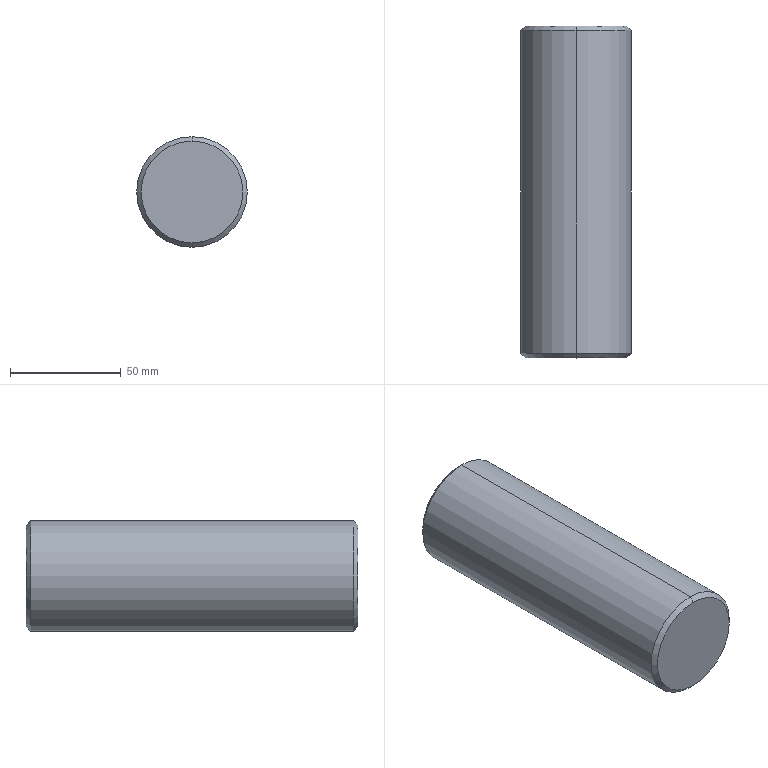Part | SolidWorks | 1 solid | 8 faces | box 50 x 150 x 50 mm | volume 293913 mm3 | cone 4 | cylinder 2 | plane 2 | commonest cylinder face diameters 50 x2
STEP:
#1=CARTESIAN_POINT('',(0.,0.,-23.));
#2=VERTEX_POINT('',#1);
#3=CARTESIAN_POINT('',(0.,0.,23.));
#4=VERTEX_POINT('',#3);
#5=CARTESIAN_POINT('',(0.,0.,0.));
#6=DIRECTION('',(0.,-1.,0.));
#7=DIRECTION('',(0.,0.,-1.));
#8=AXIS2_PLACEMENT_3D('',#5,#6,#7);
#9=CIRCLE('',#8,23.);
#10=EDGE_CURVE('',#2,#4,#9,.T.);
#11=ORIENTED_EDGE('',*,*,#10,.F.);
#12=CARTESIAN_POINT('',(0.,2.,-25.));
#13=VERTEX_POINT('',#12);
#14=CARTESIAN_POINT('',(0.,0.,-23.));
#15=DIRECTION('',(0.,0.7071,-0.7071));
#16=VECTOR('',#15,1000.);
#17=LINE('',#14,#16);
#18=EDGE_CURVE('',#2,#13,#17,.T.);
#19=ORIENTED_EDGE('',*,*,#18,.T.);
#20=CARTESIAN_POINT('',(0.,2.,25.));
#21=VERTEX_POINT('',#20);
#22=CARTESIAN_POINT('',(0.,2.,0.));
#23=DIRECTION('',(0.,-1.,0.));
#24=DIRECTION('',(0.,0.,-1.));
#25=AXIS2_PLACEMENT_3D('',#22,#23,#24);
#26=CIRCLE('',#25,25.);
#27=EDGE_CURVE('',#13,#21,#26,.T.);
#28=ORIENTED_EDGE('',*,*,#27,.T.);
#29=CARTESIAN_POINT('',(0.,0.,23.));
#30=DIRECTION('',(0.,0.7071,0.7071));
#31=VECTOR('',#30,1000.);
#32=LINE('',#29,#31);
#33=EDGE_CURVE('',#4,#21,#32,.T.);
#34=ORIENTED_EDGE('',*,*,#33,.F.);
#35=EDGE_LOOP('',(#11,#19,#28,#34));
#36=FACE_OUTER_BOUND('',#35,.T.);
#37=CARTESIAN_POINT('',(0.,0.,0.));
#38=DIRECTION('',(0.,1.,0.));
#39=DIRECTION('',(0.,0.,1.));
#40=AXIS2_PLACEMENT_3D('',#37,#38,#39);
#41=CONICAL_SURFACE('',#40,23.,0.7854);
#42=ADVANCED_FACE('',(#36),#41,.T.);
#43=CARTESIAN_POINT('',(0.,148.,-25.));
#44=VERTEX_POINT('',#43);
#45=CARTESIAN_POINT('',(0.,148.,25.));
#46=VERTEX_POINT('',#45);
#47=CARTESIAN_POINT('',(0.,148.,0.));
#48=DIRECTION('',(0.,-1.,0.));
#49=DIRECTION('',(0.,0.,-1.));
#50=AXIS2_PLACEMENT_3D('',#47,#48,#49);
#51=CIRCLE('',#50,25.);
#52=EDGE_CURVE('',#44,#46,#51,.T.);
#53=ORIENTED_EDGE('',*,*,#52,.T.);
#54=CARTESIAN_POINT('',(0.,0.,25.));
#55=DIRECTION('',(0.,-1.,0.));
#56=VECTOR('',#55,1000.);
#57=LINE('',#54,#56);
#58=EDGE_CURVE('',#46,#21,#57,.T.);
#59=ORIENTED_EDGE('',*,*,#58,.T.);
#60=ORIENTED_EDGE('',*,*,#27,.F.);
#61=CARTESIAN_POINT('',(0.,0.,-25.));
#62=DIRECTION('',(0.,-1.,0.));
#63=VECTOR('',#62,1000.);
#64=LINE('',#61,#63);
#65=EDGE_CURVE('',#44,#13,#64,.T.);
#66=ORIENTED_EDGE('',*,*,#65,.F.);
#67=EDGE_LOOP('',(#53,#59,#60,#66));
#68=FACE_OUTER_BOUND('',#67,.T.);
#69=CARTESIAN_POINT('',(0.,0.,0.));
#70=DIRECTION('',(0.,-1.,0.));
#71=DIRECTION('',(0.,0.,-1.));
#72=AXIS2_PLACEMENT_3D('',#69,#70,#71);
#73=CYLINDRICAL_SURFACE('',#72,25.);
#74=ADVANCED_FACE('',(#68),#73,.T.);
#75=CARTESIAN_POINT('',(0.,150.,-23.));
#76=VERTEX_POINT('',#75);
#77=CARTESIAN_POINT('',(0.,150.,23.));
#78=VERTEX_POINT('',#77);
#79=CARTESIAN_POINT('',(0.,150.,0.));
#80=DIRECTION('',(0.,-1.,0.));
#81=DIRECTION('',(0.,0.,-1.));
#82=AXIS2_PLACEMENT_3D('',#79,#80,#81);
#83=CIRCLE('',#82,23.);
#84=EDGE_CURVE('',#76,#78,#83,.T.);
#85=ORIENTED_EDGE('',*,*,#84,.T.);
#86=CARTESIAN_POINT('',(0.,148.,25.));
#87=DIRECTION('',(0.,-0.7071,0.7071));
#88=VECTOR('',#87,1000.);
#89=LINE('',#86,#88);
#90=EDGE_CURVE('',#78,#46,#89,.T.);
#91=ORIENTED_EDGE('',*,*,#90,.T.);
#92=ORIENTED_EDGE('',*,*,#52,.F.);
#93=CARTESIAN_POINT('',(0.,148.,-25.));
#94=DIRECTION('',(0.,-0.7071,-0.7071));
#95=VECTOR('',#94,1000.);
#96=LINE('',#93,#95);
#97=EDGE_CURVE('',#76,#44,#96,.T.);
#98=ORIENTED_EDGE('',*,*,#97,.F.);
#99=EDGE_LOOP('',(#85,#91,#92,#98));
#100=FACE_OUTER_BOUND('',#99,.T.);
#101=CARTESIAN_POINT('',(0.,148.,0.));
#102=DIRECTION('',(0.,-1.,0.));
#103=DIRECTION('',(0.,0.,-1.));
#104=AXIS2_PLACEMENT_3D('',#101,#102,#103);
#105=CONICAL_SURFACE('',#104,25.,0.7854);
#106=ADVANCED_FACE('',(#100),#105,.T.);
#107=ORIENTED_EDGE('',*,*,#84,.F.);
#108=CARTESIAN_POINT('',(0.,150.,0.));
#109=DIRECTION('',(0.,-1.,0.));
#110=DIRECTION('',(0.,0.,-1.));
#111=AXIS2_PLACEMENT_3D('',#108,#109,#110);
#112=CIRCLE('',#111,23.);
#113=EDGE_CURVE('',#78,#76,#112,.T.);
#114=ORIENTED_EDGE('',*,*,#113,.F.);
#115=EDGE_LOOP('',(#107,#114));
#116=FACE_OUTER_BOUND('',#115,.T.);
#117=CARTESIAN_POINT('',(0.,150.,0.));
#118=DIRECTION('',(0.,1.,0.));
#119=DIRECTION('',(0.,0.,1.));
#120=AXIS2_PLACEMENT_3D('',#117,#118,#119);
#121=PLANE('',#120);
#122=ADVANCED_FACE('',(#116),#121,.T.);
#123=ORIENTED_EDGE('',*,*,#90,.F.);
#124=ORIENTED_EDGE('',*,*,#113,.T.);
#125=ORIENTED_EDGE('',*,*,#97,.T.);
#126=CARTESIAN_POINT('',(0.,148.,0.));
#127=DIRECTION('',(0.,-1.,0.));
#128=DIRECTION('',(0.,0.,-1.));
#129=AXIS2_PLACEMENT_3D('',#126,#127,#128);
#130=CIRCLE('',#129,25.);
#131=EDGE_CURVE('',#46,#44,#130,.T.);
#132=ORIENTED_EDGE('',*,*,#131,.F.);
#133=EDGE_LOOP('',(#123,#124,#125,#132));
#134=FACE_OUTER_BOUND('',#133,.T.);
#135=CARTESIAN_POINT('',(0.,148.,0.));
#136=DIRECTION('',(0.,-1.,0.));
#137=DIRECTION('',(0.,0.,-1.));
#138=AXIS2_PLACEMENT_3D('',#135,#136,#137);
#139=CONICAL_SURFACE('',#138,25.,0.7854);
#140=ADVANCED_FACE('',(#134),#139,.T.);
#141=ORIENTED_EDGE('',*,*,#58,.F.);
#142=ORIENTED_EDGE('',*,*,#131,.T.);
#143=ORIENTED_EDGE('',*,*,#65,.T.);
#144=CARTESIAN_POINT('',(0.,2.,0.));
#145=DIRECTION('',(0.,-1.,0.));
#146=DIRECTION('',(0.,0.,-1.));
#147=AXIS2_PLACEMENT_3D('',#144,#145,#146);
#148=CIRCLE('',#147,25.);
#149=EDGE_CURVE('',#21,#13,#148,.T.);
#150=ORIENTED_EDGE('',*,*,#149,.F.);
#151=EDGE_LOOP('',(#141,#142,#143,#150));
#152=FACE_OUTER_BOUND('',#151,.T.);
#153=CARTESIAN_POINT('',(0.,0.,0.));
#154=DIRECTION('',(0.,-1.,0.));
#155=DIRECTION('',(0.,0.,-1.));
#156=AXIS2_PLACEMENT_3D('',#153,#154,#155);
#157=CYLINDRICAL_SURFACE('',#156,25.);
#158=ADVANCED_FACE('',(#152),#157,.T.);
#159=ORIENTED_EDGE('',*,*,#18,.F.);
#160=CARTESIAN_POINT('',(0.,0.,0.));
#161=DIRECTION('',(0.,-1.,0.));
#162=DIRECTION('',(0.,0.,-1.));
#163=AXIS2_PLACEMENT_3D('',#160,#161,#162);
#164=CIRCLE('',#163,23.);
#165=EDGE_CURVE('',#4,#2,#164,.T.);
#166=ORIENTED_EDGE('',*,*,#165,.F.);
#167=ORIENTED_EDGE('',*,*,#33,.T.);
#168=ORIENTED_EDGE('',*,*,#149,.T.);
#169=EDGE_LOOP('',(#159,#166,#167,#168));
#170=FACE_OUTER_BOUND('',#169,.T.);
#171=CARTESIAN_POINT('',(0.,0.,0.));
#172=DIRECTION('',(0.,1.,0.));
#173=DIRECTION('',(0.,0.,1.));
#174=AXIS2_PLACEMENT_3D('',#171,#172,#173);
#175=CONICAL_SURFACE('',#174,23.,0.7854);
#176=ADVANCED_FACE('',(#170),#175,.T.);
#177=ORIENTED_EDGE('',*,*,#165,.T.);
#178=ORIENTED_EDGE('',*,*,#10,.T.);
#179=EDGE_LOOP('',(#177,#178));
#180=FACE_OUTER_BOUND('',#179,.T.);
#181=CARTESIAN_POINT('',(0.,0.,0.));
#182=DIRECTION('',(0.,-1.,0.));
#183=DIRECTION('',(0.,0.,-1.));
#184=AXIS2_PLACEMENT_3D('',#181,#182,#183);
#185=PLANE('',#184);
#186=ADVANCED_FACE('',(#180),#185,.T.);
#187=CLOSED_SHELL('',(#42,#74,#106,#122,#140,#158,#176,#186));
#188=MANIFOLD_SOLID_BREP('',#187);
#189=CARTESIAN_POINT('',(0.,0.,0.));
#190=DIRECTION('',(0.,0.,1.));
#191=DIRECTION('',(1.,0.,0.));
#192=AXIS2_PLACEMENT_3D('',#189,#190,#191);
#193=(LENGTH_UNIT()NAMED_UNIT(*)SI_UNIT(.MILLI.,.METRE.));
#194=UNCERTAINTY_MEASURE_WITH_UNIT(LENGTH_MEASURE(0.00001),#193,'','');
#195=(NAMED_UNIT(*)PLANE_ANGLE_UNIT()SI_UNIT($,.RADIAN.));
#196=(NAMED_UNIT(*)SI_UNIT($,.STERADIAN.)SOLID_ANGLE_UNIT());
#197=(GEOMETRIC_REPRESENTATION_CONTEXT(3)GLOBAL_UNCERTAINTY_ASSIGNED_CONTEXT((#194))GLOBAL_UNIT_ASSIGNED_CONTEXT((#193,#195,#196))REPRESENTATION_CONTEXT('',''));
#198=ADVANCED_BREP_SHAPE_REPRESENTATION('',(#188,#192),#197);